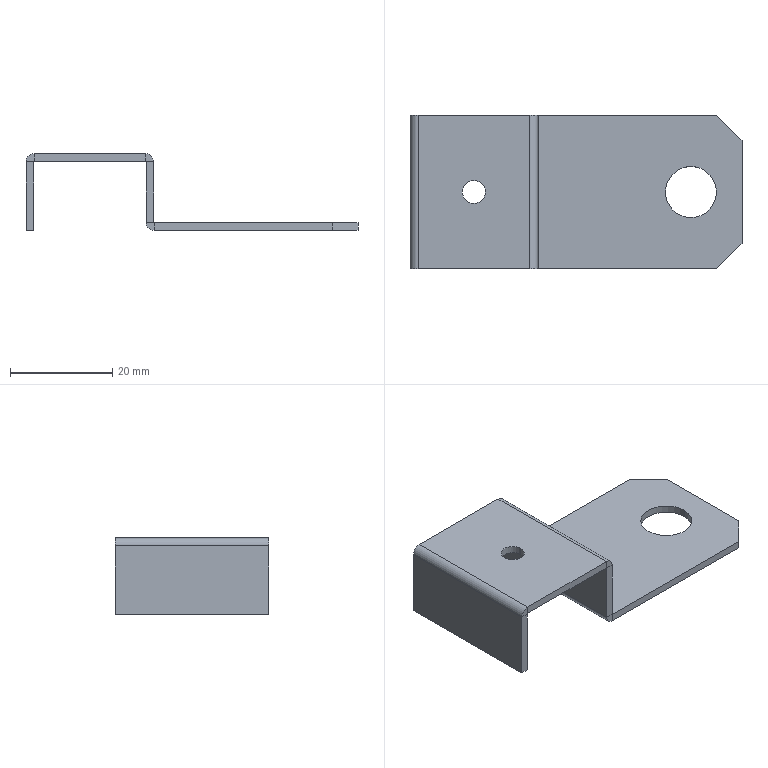Part | SolidWorks | features EdgeFlange 2, ICE 2, Chamfer 1, FlatPattern 1, SMBaseFlange 1, SheetMetal 1 | 1 solid | 36 faces | box 65 x 30 x 15 mm | volume 3912 mm3 | plane 26 | cylinder 10 | commonest cylinder face diameters 0.2 x3 3.2 x3 4.5 x2 10 x2
STEP:
#1=CARTESIAN_POINT('',(-2.25,0.,-1.5));
#2=VERTEX_POINT('',#1);
#3=CARTESIAN_POINT('',(2.25,0.,-1.5));
#4=VERTEX_POINT('',#3);
#5=CARTESIAN_POINT('',(0.,0.,-1.5));
#6=DIRECTION('',(0.,0.,1.));
#7=DIRECTION('',(1.,0.,0.));
#8=AXIS2_PLACEMENT_3D('',#5,#6,#7);
#9=CIRCLE('',#8,2.25);
#10=EDGE_CURVE('',#2,#4,#9,.T.);
#11=ORIENTED_EDGE('',*,*,#10,.F.);
#12=CARTESIAN_POINT('',(-2.25,0.,0.));
#13=VERTEX_POINT('',#12);
#14=CARTESIAN_POINT('',(-2.25,0.,-10.));
#15=DIRECTION('',(0.,0.,1.));
#16=VECTOR('',#15,1000.);
#17=LINE('',#14,#16);
#18=EDGE_CURVE('',#2,#13,#17,.T.);
#19=ORIENTED_EDGE('',*,*,#18,.T.);
#20=CARTESIAN_POINT('',(2.25,0.,0.));
#21=VERTEX_POINT('',#20);
#22=CARTESIAN_POINT('',(0.,0.,0.));
#23=DIRECTION('',(0.,0.,1.));
#24=DIRECTION('',(1.,0.,0.));
#25=AXIS2_PLACEMENT_3D('',#22,#23,#24);
#26=CIRCLE('',#25,2.25);
#27=EDGE_CURVE('',#13,#21,#26,.T.);
#28=ORIENTED_EDGE('',*,*,#27,.T.);
#29=CARTESIAN_POINT('',(2.25,0.,-10.));
#30=DIRECTION('',(0.,0.,1.));
#31=VECTOR('',#30,1000.);
#32=LINE('',#29,#31);
#33=EDGE_CURVE('',#4,#21,#32,.T.);
#34=ORIENTED_EDGE('',*,*,#33,.F.);
#35=EDGE_LOOP('',(#11,#19,#28,#34));
#36=FACE_OUTER_BOUND('',#35,.T.);
#37=CARTESIAN_POINT('',(0.,0.,-10.));
#38=DIRECTION('',(0.,0.,1.));
#39=DIRECTION('',(1.,0.,0.));
#40=AXIS2_PLACEMENT_3D('',#37,#38,#39);
#41=CYLINDRICAL_SURFACE('',#40,2.25);
#42=ADVANCED_FACE('',(#36),#41,.F.);
#43=CARTESIAN_POINT('',(37.5,0.,-15.));
#44=VERTEX_POINT('',#43);
#45=CARTESIAN_POINT('',(47.5,0.,-15.));
#46=VERTEX_POINT('',#45);
#47=CARTESIAN_POINT('',(42.5,0.,-15.));
#48=DIRECTION('',(0.,0.,1.));
#49=DIRECTION('',(1.,0.,0.));
#50=AXIS2_PLACEMENT_3D('',#47,#48,#49);
#51=CIRCLE('',#50,5.);
#52=EDGE_CURVE('',#44,#46,#51,.T.);
#53=ORIENTED_EDGE('',*,*,#52,.F.);
#54=CARTESIAN_POINT('',(37.5,0.,-13.5));
#55=VERTEX_POINT('',#54);
#56=CARTESIAN_POINT('',(37.5,0.,-23.5));
#57=DIRECTION('',(0.,0.,1.));
#58=VECTOR('',#57,1000.);
#59=LINE('',#56,#58);
#60=EDGE_CURVE('',#44,#55,#59,.T.);
#61=ORIENTED_EDGE('',*,*,#60,.T.);
#62=CARTESIAN_POINT('',(47.5,0.,-13.5));
#63=VERTEX_POINT('',#62);
#64=CARTESIAN_POINT('',(42.5,0.,-13.5));
#65=DIRECTION('',(0.,0.,1.));
#66=DIRECTION('',(1.,0.,0.));
#67=AXIS2_PLACEMENT_3D('',#64,#65,#66);
#68=CIRCLE('',#67,5.);
#69=EDGE_CURVE('',#55,#63,#68,.T.);
#70=ORIENTED_EDGE('',*,*,#69,.T.);
#71=CARTESIAN_POINT('',(47.5,0.,-23.5));
#72=DIRECTION('',(0.,0.,1.));
#73=VECTOR('',#72,1000.);
#74=LINE('',#71,#73);
#75=EDGE_CURVE('',#46,#63,#74,.T.);
#76=ORIENTED_EDGE('',*,*,#75,.F.);
#77=EDGE_LOOP('',(#53,#61,#70,#76));
#78=FACE_OUTER_BOUND('',#77,.T.);
#79=CARTESIAN_POINT('',(42.5,0.,-23.5));
#80=DIRECTION('',(0.,0.,1.));
#81=DIRECTION('',(1.,0.,0.));
#82=AXIS2_PLACEMENT_3D('',#79,#80,#81);
#83=CYLINDRICAL_SURFACE('',#82,5.);
#84=ADVANCED_FACE('',(#78),#83,.F.);
#85=CARTESIAN_POINT('',(12.5,-15.,-13.4));
#86=VERTEX_POINT('',#85);
#87=CARTESIAN_POINT('',(11.,-15.,-13.4));
#88=VERTEX_POINT('',#87);
#89=CARTESIAN_POINT('',(12.5,-15.,-13.4));
#90=DIRECTION('',(-1.,0.,0.));
#91=VECTOR('',#90,1000.);
#92=LINE('',#89,#91);
#93=EDGE_CURVE('',#86,#88,#92,.T.);
#94=ORIENTED_EDGE('',*,*,#93,.F.);
#95=CARTESIAN_POINT('',(12.5,-15.,-1.6));
#96=VERTEX_POINT('',#95);
#97=CARTESIAN_POINT('',(12.5,-15.,-1.5));
#98=DIRECTION('',(0.,0.,-1.));
#99=VECTOR('',#98,1000.);
#100=LINE('',#97,#99);
#101=EDGE_CURVE('',#96,#86,#100,.T.);
#102=ORIENTED_EDGE('',*,*,#101,.F.);
#103=CARTESIAN_POINT('',(11.,-15.,-1.6));
#104=VERTEX_POINT('',#103);
#105=CARTESIAN_POINT('',(11.,-15.,-1.6));
#106=DIRECTION('',(1.,0.,0.));
#107=VECTOR('',#106,1000.);
#108=LINE('',#105,#107);
#109=EDGE_CURVE('',#104,#96,#108,.T.);
#110=ORIENTED_EDGE('',*,*,#109,.F.);
#111=CARTESIAN_POINT('',(11.,-15.,-15.));
#112=DIRECTION('',(0.,0.,-1.));
#113=VECTOR('',#112,1000.);
#114=LINE('',#111,#113);
#115=EDGE_CURVE('',#104,#88,#114,.T.);
#116=ORIENTED_EDGE('',*,*,#115,.T.);
#117=EDGE_LOOP('',(#94,#102,#110,#116));
#118=FACE_OUTER_BOUND('',#117,.T.);
#119=CARTESIAN_POINT('',(12.5,-15.,-15.));
#120=DIRECTION('',(0.,1.,0.));
#121=DIRECTION('',(-1.,0.,0.));
#122=AXIS2_PLACEMENT_3D('',#119,#120,#121);
#123=PLANE('',#122);
#124=ADVANCED_FACE('',(#118),#123,.F.);
#125=CARTESIAN_POINT('',(12.5,15.,-13.4));
#126=VERTEX_POINT('',#125);
#127=CARTESIAN_POINT('',(11.,15.,-13.4));
#128=VERTEX_POINT('',#127);
#129=CARTESIAN_POINT('',(12.5,15.,-13.4));
#130=DIRECTION('',(-1.,0.,0.));
#131=VECTOR('',#130,1000.);
#132=LINE('',#129,#131);
#133=EDGE_CURVE('',#126,#128,#132,.T.);
#134=ORIENTED_EDGE('',*,*,#133,.T.);
#135=CARTESIAN_POINT('',(11.,15.,-1.6));
#136=VERTEX_POINT('',#135);
#137=CARTESIAN_POINT('',(11.,15.,-1.5));
#138=DIRECTION('',(0.,0.,1.));
#139=VECTOR('',#138,1000.);
#140=LINE('',#137,#139);
#141=EDGE_CURVE('',#128,#136,#140,.T.);
#142=ORIENTED_EDGE('',*,*,#141,.T.);
#143=CARTESIAN_POINT('',(12.5,15.,-1.6));
#144=VERTEX_POINT('',#143);
#145=CARTESIAN_POINT('',(12.5,15.,-1.6));
#146=DIRECTION('',(1.,0.,0.));
#147=VECTOR('',#146,1000.);
#148=LINE('',#145,#147);
#149=EDGE_CURVE('',#136,#144,#148,.T.);
#150=ORIENTED_EDGE('',*,*,#149,.T.);
#151=CARTESIAN_POINT('',(12.5,15.,-1.5));
#152=DIRECTION('',(0.,0.,1.));
#153=VECTOR('',#152,1000.);
#154=LINE('',#151,#153);
#155=EDGE_CURVE('',#126,#144,#154,.T.);
#156=ORIENTED_EDGE('',*,*,#155,.F.);
#157=EDGE_LOOP('',(#134,#142,#150,#156));
#158=FACE_OUTER_BOUND('',#157,.T.);
#159=CARTESIAN_POINT('',(12.5,15.,-1.5));
#160=DIRECTION('',(0.,-1.,0.));
#161=DIRECTION('',(1.,0.,0.));
#162=AXIS2_PLACEMENT_3D('',#159,#160,#161);
#163=PLANE('',#162);
#164=ADVANCED_FACE('',(#158),#163,.F.);
#165=CARTESIAN_POINT('',(12.5,15.,-13.4));
#166=DIRECTION('',(0.,-1.,0.));
#167=VECTOR('',#166,1000.);
#168=LINE('',#165,#167);
#169=EDGE_CURVE('',#126,#86,#168,.T.);
#170=ORIENTED_EDGE('',*,*,#169,.F.);
#171=ORIENTED_EDGE('',*,*,#155,.T.);
#172=CARTESIAN_POINT('',(12.5,15.,-1.6));
#173=DIRECTION('',(0.,1.,0.));
#174=VECTOR('',#173,1000.);
#175=LINE('',#172,#174);
#176=EDGE_CURVE('',#96,#144,#175,.T.);
#177=ORIENTED_EDGE('',*,*,#176,.F.);
#178=ORIENTED_EDGE('',*,*,#101,.T.);
#179=EDGE_LOOP('',(#170,#171,#177,#178));
#180=FACE_OUTER_BOUND('',#179,.T.);
#181=CARTESIAN_POINT('',(12.5,-15.,-1.5));
#182=DIRECTION('',(-1.,0.,0.));
#183=DIRECTION('',(0.,0.,1.));
#184=AXIS2_PLACEMENT_3D('',#181,#182,#183);
#185=PLANE('',#184);
#186=ADVANCED_FACE('',(#180),#185,.F.);
#187=ORIENTED_EDGE('',*,*,#141,.F.);
#188=CARTESIAN_POINT('',(11.,15.,-13.4));
#189=DIRECTION('',(0.,-1.,0.));
#190=VECTOR('',#189,1000.);
#191=LINE('',#188,#190);
#192=EDGE_CURVE('',#128,#88,#191,.T.);
#193=ORIENTED_EDGE('',*,*,#192,.T.);
#194=ORIENTED_EDGE('',*,*,#115,.F.);
#195=CARTESIAN_POINT('',(11.,15.,-1.6));
#196=DIRECTION('',(0.,-1.,0.));
#197=VECTOR('',#196,1000.);
#198=LINE('',#195,#197);
#199=EDGE_CURVE('',#136,#104,#198,.T.);
#200=ORIENTED_EDGE('',*,*,#199,.F.);
#201=EDGE_LOOP('',(#187,#193,#194,#200));
#202=FACE_OUTER_BOUND('',#201,.T.);
#203=CARTESIAN_POINT('',(11.,-15.,-1.5));
#204=DIRECTION('',(-1.,0.,0.));
#205=DIRECTION('',(0.,0.,1.));
#206=AXIS2_PLACEMENT_3D('',#203,#204,#205);
#207=PLANE('',#206);
#208=ADVANCED_FACE('',(#202),#207,.T.);
#209=CARTESIAN_POINT('',(0.,0.,-1.5));
#210=DIRECTION('',(0.,0.,1.));
#211=DIRECTION('',(1.,0.,0.));
#212=AXIS2_PLACEMENT_3D('',#209,#210,#211);
#213=CIRCLE('',#212,2.25);
#214=EDGE_CURVE('',#4,#2,#213,.T.);
#215=ORIENTED_EDGE('',*,*,#214,.T.);
#216=ORIENTED_EDGE('',*,*,#10,.T.);
#217=EDGE_LOOP('',(#215,#216));
#218=FACE_BOUND('',#217,.T.);
#219=CARTESIAN_POINT('',(-10.9,15.,-1.5));
#220=VERTEX_POINT('',#219);
#221=CARTESIAN_POINT('',(-10.9,-15.,-1.5));
#222=VERTEX_POINT('',#221);
#223=CARTESIAN_POINT('',(-10.9,15.,-1.5));
#224=DIRECTION('',(0.,-1.,0.));
#225=VECTOR('',#224,1000.);
#226=LINE('',#223,#225);
#227=EDGE_CURVE('',#220,#222,#226,.T.);
#228=ORIENTED_EDGE('',*,*,#227,.F.);
#229=CARTESIAN_POINT('',(10.9,15.,-1.5));
#230=VERTEX_POINT('',#229);
#231=CARTESIAN_POINT('',(-12.5,15.,-1.5));
#232=DIRECTION('',(-1.,0.,0.));
#233=VECTOR('',#232,1000.);
#234=LINE('',#231,#233);
#235=EDGE_CURVE('',#230,#220,#234,.T.);
#236=ORIENTED_EDGE('',*,*,#235,.F.);
#237=CARTESIAN_POINT('',(10.9,-15.,-1.5));
#238=VERTEX_POINT('',#237);
#239=CARTESIAN_POINT('',(10.9,-15.,-1.5));
#240=DIRECTION('',(0.,1.,0.));
#241=VECTOR('',#240,1000.);
#242=LINE('',#239,#241);
#243=EDGE_CURVE('',#238,#230,#242,.T.);
#244=ORIENTED_EDGE('',*,*,#243,.F.);
#245=CARTESIAN_POINT('',(-12.5,-15.,-1.5));
#246=DIRECTION('',(1.,0.,0.));
#247=VECTOR('',#246,1000.);
#248=LINE('',#245,#247);
#249=EDGE_CURVE('',#222,#238,#248,.T.);
#250=ORIENTED_EDGE('',*,*,#249,.F.);
#251=EDGE_LOOP('',(#228,#236,#244,#250));
#252=FACE_OUTER_BOUND('',#251,.T.);
#253=CARTESIAN_POINT('',(12.5,-15.,-1.5));
#254=DIRECTION('',(0.,0.,1.));
#255=DIRECTION('',(1.,0.,0.));
#256=AXIS2_PLACEMENT_3D('',#253,#254,#255);
#257=PLANE('',#256);
#258=ADVANCED_FACE('',(#218,#252),#257,.F.);
#259=CARTESIAN_POINT('',(0.,0.,0.));
#260=DIRECTION('',(0.,0.,1.));
#261=DIRECTION('',(1.,0.,0.));
#262=AXIS2_PLACEMENT_3D('',#259,#260,#261);
#263=CIRCLE('',#262,2.25);
#264=EDGE_CURVE('',#21,#13,#263,.T.);
#265=ORIENTED_EDGE('',*,*,#264,.F.);
#266=ORIENTED_EDGE('',*,*,#27,.F.);
#267=EDGE_LOOP('',(#265,#266));
#268=FACE_BOUND('',#267,.T.);
#269=CARTESIAN_POINT('',(10.9,15.,0.));
#270=VERTEX_POINT('',#269);
#271=CARTESIAN_POINT('',(-10.9,15.,0.));
#272=VERTEX_POINT('',#271);
#273=CARTESIAN_POINT('',(-12.5,15.,0.));
#274=DIRECTION('',(-1.,0.,0.));
#275=VECTOR('',#274,1000.);
#276=LINE('',#273,#275);
#277=EDGE_CURVE('',#270,#272,#276,.T.);
#278=ORIENTED_EDGE('',*,*,#277,.T.);
#279=CARTESIAN_POINT('',(-10.9,-15.,0.));
#280=VERTEX_POINT('',#279);
#281=CARTESIAN_POINT('',(-10.9,15.,0.));
#282=DIRECTION('',(0.,-1.,0.));
#283=VECTOR('',#282,1000.);
#284=LINE('',#281,#283);
#285=EDGE_CURVE('',#272,#280,#284,.T.);
#286=ORIENTED_EDGE('',*,*,#285,.T.);
#287=CARTESIAN_POINT('',(10.9,-15.,0.));
#288=VERTEX_POINT('',#287);
#289=CARTESIAN_POINT('',(-12.5,-15.,0.));
#290=DIRECTION('',(1.,0.,0.));
#291=VECTOR('',#290,1000.);
#292=LINE('',#289,#291);
#293=EDGE_CURVE('',#280,#288,#292,.T.);
#294=ORIENTED_EDGE('',*,*,#293,.T.);
#295=CARTESIAN_POINT('',(10.9,-15.,0.));
#296=DIRECTION('',(0.,1.,0.));
#297=VECTOR('',#296,1000.);
#298=LINE('',#295,#297);
#299=EDGE_CURVE('',#288,#270,#298,.T.);
#300=ORIENTED_EDGE('',*,*,#299,.T.);
#301=EDGE_LOOP('',(#278,#286,#294,#300));
#302=FACE_OUTER_BOUND('',#301,.T.);
#303=CARTESIAN_POINT('',(12.5,-15.,0.));
#304=DIRECTION('',(0.,0.,1.));
#305=DIRECTION('',(1.,0.,0.));
#306=AXIS2_PLACEMENT_3D('',#303,#304,#305);
#307=PLANE('',#306);
#308=ADVANCED_FACE('',(#268,#302),#307,.T.);
#309=ORIENTED_EDGE('',*,*,#235,.T.);
#310=CARTESIAN_POINT('',(-10.9,15.,-1.5));
#311=DIRECTION('',(0.,0.,1.));
#312=VECTOR('',#311,1000.);
#313=LINE('',#310,#312);
#314=EDGE_CURVE('',#220,#272,#313,.T.);
#315=ORIENTED_EDGE('',*,*,#314,.T.);
#316=ORIENTED_EDGE('',*,*,#277,.F.);
#317=CARTESIAN_POINT('',(10.9,15.,-1.5));
#318=DIRECTION('',(0.,0.,1.));
#319=VECTOR('',#318,1000.);
#320=LINE('',#317,#319);
#321=EDGE_CURVE('',#230,#270,#320,.T.);
#322=ORIENTED_EDGE('',*,*,#321,.F.);
#323=EDGE_LOOP('',(#309,#315,#316,#322));
#324=FACE_OUTER_BOUND('',#323,.T.);
#325=CARTESIAN_POINT('',(-12.5,15.,-1.5));
#326=DIRECTION('',(0.,1.,0.));
#327=DIRECTION('',(0.,0.,1.));
#328=AXIS2_PLACEMENT_3D('',#325,#326,#327);
#329=PLANE('',#328);
#330=ADVANCED_FACE('',(#324),#329,.T.);
#331=CARTESIAN_POINT('',(-10.9,-15.,-1.5));
#332=DIRECTION('',(0.,0.,1.));
#333=VECTOR('',#332,1000.);
#334=LINE('',#331,#333);
#335=EDGE_CURVE('',#222,#280,#334,.T.);
#336=ORIENTED_EDGE('',*,*,#335,.F.);
#337=ORIENTED_EDGE('',*,*,#249,.T.);
#338=CARTESIAN_POINT('',(10.9,-15.,-1.5));
#339=DIRECTION('',(0.,0.,1.));
#340=VECTOR('',#339,1000.);
#341=LINE('',#338,#340);
#342=EDGE_CURVE('',#238,#288,#341,.T.);
#343=ORIENTED_EDGE('',*,*,#342,.T.);
#344=ORIENTED_EDGE('',*,*,#293,.F.);
#345=EDGE_LOOP('',(#336,#337,#343,#344));
#346=FACE_OUTER_BOUND('',#345,.T.);
#347=CARTESIAN_POINT('',(-12.5,-15.,-1.5));
#348=DIRECTION('',(0.,-1.,0.));
#349=DIRECTION('',(0.,0.,-1.));
#350=AXIS2_PLACEMENT_3D('',#347,#348,#349);
#351=PLANE('',#350);
#352=ADVANCED_FACE('',(#346),#351,.T.);
#353=ORIENTED_EDGE('',*,*,#149,.F.);
#354=CARTESIAN_POINT('',(10.9,15.,-1.6));
#355=DIRECTION('',(0.,1.,0.));
#356=DIRECTION('',(0.,0.,-1.));
#357=AXIS2_PLACEMENT_3D('',#354,#355,#356);
#358=CIRCLE('',#357,0.1);
#359=EDGE_CURVE('',#230,#136,#358,.T.);
#360=ORIENTED_EDGE('',*,*,#359,.F.);
#361=ORIENTED_EDGE('',*,*,#321,.T.);
#362=CARTESIAN_POINT('',(10.9,15.,-1.6));
#363=DIRECTION('',(0.,1.,0.));
#364=DIRECTION('',(0.,0.,-1.));
#365=AXIS2_PLACEMENT_3D('',#362,#363,#364);
#366=CIRCLE('',#365,1.6);
#367=EDGE_CURVE('',#270,#144,#366,.T.);
#368=ORIENTED_EDGE('',*,*,#367,.T.);
#369=EDGE_LOOP('',(#353,#360,#361,#368));
#370=FACE_OUTER_BOUND('',#369,.T.);
#371=CARTESIAN_POINT('',(10.9,15.,-1.6));
#372=DIRECTION('',(0.,1.,0.));
#373=DIRECTION('',(0.,0.,1.));
#374=AXIS2_PLACEMENT_3D('',#371,#372,#373);
#375=PLANE('',#374);
#376=ADVANCED_FACE('',(#370),#375,.T.);
#377=CARTESIAN_POINT('',(10.9,-15.,-1.6));
#378=DIRECTION('',(0.,-1.,0.));
#379=DIRECTION('',(0.,0.,-1.));
#380=AXIS2_PLACEMENT_3D('',#377,#378,#379);
#381=CIRCLE('',#380,0.1);
#382=EDGE_CURVE('',#104,#238,#381,.T.);
#383=ORIENTED_EDGE('',*,*,#382,.F.);
#384=ORIENTED_EDGE('',*,*,#109,.T.);
#385=CARTESIAN_POINT('',(10.9,-15.,-1.6));
#386=DIRECTION('',(0.,-1.,0.));
#387=DIRECTION('',(0.,0.,-1.));
#388=AXIS2_PLACEMENT_3D('',#385,#386,#387);
#389=CIRCLE('',#388,1.6);
#390=EDGE_CURVE('',#96,#288,#389,.T.);
#391=ORIENTED_EDGE('',*,*,#390,.T.);
#392=ORIENTED_EDGE('',*,*,#342,.F.);
#393=EDGE_LOOP('',(#383,#384,#391,#392));
#394=FACE_OUTER_BOUND('',#393,.T.);
#395=CARTESIAN_POINT('',(10.9,-15.,-1.6));
#396=DIRECTION('',(0.,1.,0.));
#397=DIRECTION('',(0.,0.,1.));
#398=AXIS2_PLACEMENT_3D('',#395,#396,#397);
#399=PLANE('',#398);
#400=ADVANCED_FACE('',(#394),#399,.F.);
#401=ORIENTED_EDGE('',*,*,#299,.F.);
#402=ORIENTED_EDGE('',*,*,#390,.F.);
#403=ORIENTED_EDGE('',*,*,#176,.T.);
#404=ORIENTED_EDGE('',*,*,#367,.F.);
#405=EDGE_LOOP('',(#401,#402,#403,#404));
#406=FACE_OUTER_BOUND('',#405,.T.);
#407=CARTESIAN_POINT('',(10.9,-15.,-1.6));
#408=DIRECTION('',(0.,-1.,0.));
#409=DIRECTION('',(1.,0.,0.));
#410=AXIS2_PLACEMENT_3D('',#407,#408,#409);
#411=CYLINDRICAL_SURFACE('',#410,1.6);
#412=ADVANCED_FACE('',(#406),#411,.T.);
#413=ORIENTED_EDGE('',*,*,#243,.T.);
#414=ORIENTED_EDGE('',*,*,#359,.T.);
#415=ORIENTED_EDGE('',*,*,#199,.T.);
#416=ORIENTED_EDGE('',*,*,#382,.T.);
#417=EDGE_LOOP('',(#413,#414,#415,#416));
#418=FACE_OUTER_BOUND('',#417,.T.);
#419=CARTESIAN_POINT('',(10.9,-15.,-1.6));
#420=DIRECTION('',(0.,-1.,0.));
#421=DIRECTION('',(1.,0.,0.));
#422=AXIS2_PLACEMENT_3D('',#419,#420,#421);
#423=CYLINDRICAL_SURFACE('',#422,0.1);
#424=ADVANCED_FACE('',(#418),#423,.F.);
#425=CARTESIAN_POINT('',(-11.,-15.,-1.6));
#426=VERTEX_POINT('',#425);
#427=CARTESIAN_POINT('',(-12.5,-15.,-1.6));
#428=VERTEX_POINT('',#427);
#429=CARTESIAN_POINT('',(-12.5,-15.,-1.6));
#430=DIRECTION('',(-1.,0.,0.));
#431=VECTOR('',#430,1000.);
#432=LINE('',#429,#431);
#433=EDGE_CURVE('',#426,#428,#432,.T.);
#434=ORIENTED_EDGE('',*,*,#433,.F.);
#435=CARTESIAN_POINT('',(-10.9,-15.,-1.6));
#436=DIRECTION('',(0.,-1.,0.));
#437=DIRECTION('',(0.,0.,1.));
#438=AXIS2_PLACEMENT_3D('',#435,#436,#437);
#439=CIRCLE('',#438,0.1);
#440=EDGE_CURVE('',#222,#426,#439,.T.);
#441=ORIENTED_EDGE('',*,*,#440,.F.);
#442=ORIENTED_EDGE('',*,*,#335,.T.);
#443=CARTESIAN_POINT('',(-10.9,-15.,-1.6));
#444=DIRECTION('',(0.,-1.,0.));
#445=DIRECTION('',(0.,0.,1.));
#446=AXIS2_PLACEMENT_3D('',#443,#444,#445);
#447=CIRCLE('',#446,1.6);
#448=EDGE_CURVE('',#280,#428,#447,.T.);
#449=ORIENTED_EDGE('',*,*,#448,.T.);
#450=EDGE_LOOP('',(#434,#441,#442,#449));
#451=FACE_OUTER_BOUND('',#450,.T.);
#452=CARTESIAN_POINT('',(-10.9,-15.,-1.6));
#453=DIRECTION('',(0.,-1.,0.));
#454=DIRECTION('',(0.,0.,-1.));
#455=AXIS2_PLACEMENT_3D('',#452,#453,#454);
#456=PLANE('',#455);
#457=ADVANCED_FACE('',(#451),#456,.T.);
#458=CARTESIAN_POINT('',(-11.,15.,-1.6));
#459=VERTEX_POINT('',#458);
#460=CARTESIAN_POINT('',(-10.9,15.,-1.6));
#461=DIRECTION('',(0.,1.,0.));
#462=DIRECTION('',(0.,0.,1.));
#463=AXIS2_PLACEMENT_3D('',#460,#461,#462);
#464=CIRCLE('',#463,0.1);
#465=EDGE_CURVE('',#459,#220,#464,.T.);
#466=ORIENTED_EDGE('',*,*,#465,.F.);
#467=CARTESIAN_POINT('',(-12.5,15.,-1.6));
#468=VERTEX_POINT('',#467);
#469=CARTESIAN_POINT('',(-11.,15.,-1.6));
#470=DIRECTION('',(-1.,0.,0.));
#471=VECTOR('',#470,1000.);
#472=LINE('',#469,#471);
#473=EDGE_CURVE('',#459,#468,#472,.T.);
#474=ORIENTED_EDGE('',*,*,#473,.T.);
#475=CARTESIAN_POINT('',(-10.9,15.,-1.6));
#476=DIRECTION('',(0.,1.,0.));
#477=DIRECTION('',(0.,0.,1.));
#478=AXIS2_PLACEMENT_3D('',#475,#476,#477);
#479=CIRCLE('',#478,1.6);
#480=EDGE_CURVE('',#468,#272,#479,.T.);
#481=ORIENTED_EDGE('',*,*,#480,.T.);
#482=ORIENTED_EDGE('',*,*,#314,.F.);
#483=EDGE_LOOP('',(#466,#474,#481,#482));
#484=FACE_OUTER_BOUND('',#483,.T.);
#485=CARTESIAN_POINT('',(-10.9,15.,-1.6));
#486=DIRECTION('',(0.,-1.,0.));
#487=DIRECTION('',(0.,0.,-1.));
#488=AXIS2_PLACEMENT_3D('',#485,#486,#487);
#489=PLANE('',#488);
#490=ADVANCED_FACE('',(#484),#489,.F.);
#491=ORIENTED_EDGE('',*,*,#285,.F.);
#492=ORIENTED_EDGE('',*,*,#480,.F.);
#493=CARTESIAN_POINT('',(-12.5,-15.,-1.6));
#494=DIRECTION('',(0.,-1.,0.));
#495=VECTOR('',#494,1000.);
#496=LINE('',#493,#495);
#497=EDGE_CURVE('',#468,#428,#496,.T.);
#498=ORIENTED_EDGE('',*,*,#497,.T.);
#499=ORIENTED_EDGE('',*,*,#448,.F.);
#500=EDGE_LOOP('',(#491,#492,#498,#499));
#501=FACE_OUTER_BOUND('',#500,.T.);
#502=CARTESIAN_POINT('',(-10.9,15.,-1.6));
#503=DIRECTION('',(0.,1.,0.));
#504=DIRECTION('',(-1.,0.,0.));
#505=AXIS2_PLACEMENT_3D('',#502,#503,#504);
#506=CYLINDRICAL_SURFACE('',#505,1.6);
#507=ADVANCED_FACE('',(#501),#506,.T.);
#508=ORIENTED_EDGE('',*,*,#227,.T.);
#509=ORIENTED_EDGE('',*,*,#440,.T.);
#510=CARTESIAN_POINT('',(-11.,-15.,-1.6));
#511=DIRECTION('',(0.,1.,0.));
#512=VECTOR('',#511,1000.);
#513=LINE('',#510,#512);
#514=EDGE_CURVE('',#426,#459,#513,.T.);
#515=ORIENTED_EDGE('',*,*,#514,.T.);
#516=ORIENTED_EDGE('',*,*,#465,.T.);
#517=EDGE_LOOP('',(#508,#509,#515,#516));
#518=FACE_OUTER_BOUND('',#517,.T.);
#519=CARTESIAN_POINT('',(-10.9,15.,-1.6));
#520=DIRECTION('',(0.,1.,0.));
#521=DIRECTION('',(-1.,0.,0.));
#522=AXIS2_PLACEMENT_3D('',#519,#520,#521);
#523=CYLINDRICAL_SURFACE('',#522,0.1);
#524=ADVANCED_FACE('',(#518),#523,.F.);
#525=ORIENTED_EDGE('',*,*,#473,.F.);
#526=CARTESIAN_POINT('',(-11.,15.,-15.));
#527=VERTEX_POINT('',#526);
#528=CARTESIAN_POINT('',(-11.,15.,-15.));
#529=DIRECTION('',(0.,0.,-1.));
#530=VECTOR('',#529,1000.);
#531=LINE('',#528,#530);
#532=EDGE_CURVE('',#459,#527,#531,.T.);
#533=ORIENTED_EDGE('',*,*,#532,.T.);
#534=CARTESIAN_POINT('',(-12.5,15.,-15.));
#535=VERTEX_POINT('',#534);
#536=CARTESIAN_POINT('',(-12.5,15.,-15.));
#537=DIRECTION('',(1.,0.,0.));
#538=VECTOR('',#537,1000.);
#539=LINE('',#536,#538);
#540=EDGE_CURVE('',#535,#527,#539,.T.);
#541=ORIENTED_EDGE('',*,*,#540,.F.);
#542=CARTESIAN_POINT('',(-12.5,15.,-1.5));
#543=DIRECTION('',(0.,0.,-1.));
#544=VECTOR('',#543,1000.);
#545=LINE('',#542,#544);
#546=EDGE_CURVE('',#468,#535,#545,.T.);
#547=ORIENTED_EDGE('',*,*,#546,.F.);
#548=EDGE_LOOP('',(#525,#533,#541,#547));
#549=FACE_OUTER_BOUND('',#548,.T.);
#550=CARTESIAN_POINT('',(-12.5,15.,-15.));
#551=DIRECTION('',(0.,-1.,0.));
#552=DIRECTION('',(1.,0.,0.));
#553=AXIS2_PLACEMENT_3D('',#550,#551,#552);
#554=PLANE('',#553);
#555=ADVANCED_FACE('',(#549),#554,.F.);
#556=ORIENTED_EDGE('',*,*,#433,.T.);
#557=CARTESIAN_POINT('',(-12.5,-15.,-15.));
#558=VERTEX_POINT('',#557);
#559=CARTESIAN_POINT('',(-12.5,-15.,-1.5));
#560=DIRECTION('',(0.,0.,1.));
#561=VECTOR('',#560,1000.);
#562=LINE('',#559,#561);
#563=EDGE_CURVE('',#558,#428,#562,.T.);
#564=ORIENTED_EDGE('',*,*,#563,.F.);
#565=CARTESIAN_POINT('',(-11.,-15.,-15.));
#566=VERTEX_POINT('',#565);
#567=CARTESIAN_POINT('',(-12.5,-15.,-15.));
#568=DIRECTION('',(1.,0.,0.));
#569=VECTOR('',#568,1000.);
#570=LINE('',#567,#569);
#571=EDGE_CURVE('',#558,#566,#570,.T.);
#572=ORIENTED_EDGE('',*,*,#571,.T.);
#573=CARTESIAN_POINT('',(-11.,-15.,-1.5));
#574=DIRECTION('',(0.,0.,1.));
#575=VECTOR('',#574,1000.);
#576=LINE('',#573,#575);
#577=EDGE_CURVE('',#566,#426,#576,.T.);
#578=ORIENTED_EDGE('',*,*,#577,.T.);
#579=EDGE_LOOP('',(#556,#564,#572,#578));
#580=FACE_OUTER_BOUND('',#579,.T.);
#581=CARTESIAN_POINT('',(-12.5,-15.,-1.5));
#582=DIRECTION('',(0.,1.,0.));
#583=DIRECTION('',(-1.,0.,0.));
#584=AXIS2_PLACEMENT_3D('',#581,#582,#583);
#585=PLANE('',#584);
#586=ADVANCED_FACE('',(#580),#585,.F.);
#587=ORIENTED_EDGE('',*,*,#497,.F.);
#588=ORIENTED_EDGE('',*,*,#546,.T.);
#589=CARTESIAN_POINT('',(-12.5,15.,-15.));
#590=DIRECTION('',(0.,-1.,0.));
#591=VECTOR('',#590,1000.);
#592=LINE('',#589,#591);
#593=EDGE_CURVE('',#535,#558,#592,.T.);
#594=ORIENTED_EDGE('',*,*,#593,.T.);
#595=ORIENTED_EDGE('',*,*,#563,.T.);
#596=EDGE_LOOP('',(#587,#588,#594,#595));
#597=FACE_OUTER_BOUND('',#596,.T.);
#598=CARTESIAN_POINT('',(-12.5,15.,-1.5));
#599=DIRECTION('',(1.,0.,0.));
#600=DIRECTION('',(0.,0.,-1.));
#601=AXIS2_PLACEMENT_3D('',#598,#599,#600);
#602=PLANE('',#601);
#603=ADVANCED_FACE('',(#597),#602,.F.);
#604=ORIENTED_EDGE('',*,*,#532,.F.);
#605=ORIENTED_EDGE('',*,*,#514,.F.);
#606=ORIENTED_EDGE('',*,*,#577,.F.);
#607=CARTESIAN_POINT('',(-11.,-15.,-15.));
#608=DIRECTION('',(0.,-1.,0.));
#609=VECTOR('',#608,1000.);
#610=LINE('',#607,#609);
#611=EDGE_CURVE('',#527,#566,#610,.T.);
#612=ORIENTED_EDGE('',*,*,#611,.F.);
#613=EDGE_LOOP('',(#604,#605,#606,#612));
#614=FACE_OUTER_BOUND('',#613,.T.);
#615=CARTESIAN_POINT('',(-11.,15.,-1.5));
#616=DIRECTION('',(1.,0.,0.));
#617=DIRECTION('',(0.,0.,-1.));
#618=AXIS2_PLACEMENT_3D('',#615,#616,#617);
#619=PLANE('',#618);
#620=ADVANCED_FACE('',(#614),#619,.T.);
#621=ORIENTED_EDGE('',*,*,#611,.T.);
#622=ORIENTED_EDGE('',*,*,#571,.F.);
#623=ORIENTED_EDGE('',*,*,#593,.F.);
#624=ORIENTED_EDGE('',*,*,#540,.T.);
#625=EDGE_LOOP('',(#621,#622,#623,#624));
#626=FACE_OUTER_BOUND('',#625,.T.);
#627=CARTESIAN_POINT('',(-12.5,-15.,-15.));
#628=DIRECTION('',(0.,0.,1.));
#629=DIRECTION('',(1.,0.,0.));
#630=AXIS2_PLACEMENT_3D('',#627,#628,#629);
#631=PLANE('',#630);
#632=ADVANCED_FACE('',(#626),#631,.F.);
#633=CARTESIAN_POINT('',(12.6,-15.,-13.5));
#634=VERTEX_POINT('',#633);
#635=CARTESIAN_POINT('',(12.6,-15.,-15.));
#636=VERTEX_POINT('',#635);
#637=CARTESIAN_POINT('',(12.6,-15.,-15.));
#638=DIRECTION('',(0.,0.,-1.));
#639=VECTOR('',#638,1000.);
#640=LINE('',#637,#639);
#641=EDGE_CURVE('',#634,#636,#640,.T.);
#642=ORIENTED_EDGE('',*,*,#641,.F.);
#643=CARTESIAN_POINT('',(12.6,-15.,-13.4));
#644=DIRECTION('',(0.,-1.,0.));
#645=DIRECTION('',(0.,0.,1.));
#646=AXIS2_PLACEMENT_3D('',#643,#644,#645);
#647=CIRCLE('',#646,0.1);
#648=EDGE_CURVE('',#86,#634,#647,.T.);
#649=ORIENTED_EDGE('',*,*,#648,.F.);
#650=ORIENTED_EDGE('',*,*,#93,.T.);
#651=CARTESIAN_POINT('',(12.6,-15.,-13.4));
#652=DIRECTION('',(0.,-1.,0.));
#653=DIRECTION('',(0.,0.,1.));
#654=AXIS2_PLACEMENT_3D('',#651,#652,#653);
#655=CIRCLE('',#654,1.6);
#656=EDGE_CURVE('',#88,#636,#655,.T.);
#657=ORIENTED_EDGE('',*,*,#656,.T.);
#658=EDGE_LOOP('',(#642,#649,#650,#657));
#659=FACE_OUTER_BOUND('',#658,.T.);
#660=CARTESIAN_POINT('',(12.6,-15.,-13.4));
#661=DIRECTION('',(0.,-1.,0.));
#662=DIRECTION('',(0.,0.,-1.));
#663=AXIS2_PLACEMENT_3D('',#660,#661,#662);
#664=PLANE('',#663);
#665=ADVANCED_FACE('',(#659),#664,.T.);
#666=CARTESIAN_POINT('',(12.6,15.,-13.5));
#667=VERTEX_POINT('',#666);
#668=CARTESIAN_POINT('',(12.6,15.,-13.4));
#669=DIRECTION('',(0.,1.,0.));
#670=DIRECTION('',(0.,0.,1.));
#671=AXIS2_PLACEMENT_3D('',#668,#669,#670);
#672=CIRCLE('',#671,0.1);
#673=EDGE_CURVE('',#667,#126,#672,.T.);
#674=ORIENTED_EDGE('',*,*,#673,.F.);
#675=CARTESIAN_POINT('',(12.6,15.,-15.));
#676=VERTEX_POINT('',#675);
#677=CARTESIAN_POINT('',(12.6,15.,-13.5));
#678=DIRECTION('',(0.,0.,-1.));
#679=VECTOR('',#678,1000.);
#680=LINE('',#677,#679);
#681=EDGE_CURVE('',#667,#676,#680,.T.);
#682=ORIENTED_EDGE('',*,*,#681,.T.);
#683=CARTESIAN_POINT('',(12.6,15.,-13.4));
#684=DIRECTION('',(0.,1.,0.));
#685=DIRECTION('',(0.,0.,1.));
#686=AXIS2_PLACEMENT_3D('',#683,#684,#685);
#687=CIRCLE('',#686,1.6);
#688=EDGE_CURVE('',#676,#128,#687,.T.);
#689=ORIENTED_EDGE('',*,*,#688,.T.);
#690=ORIENTED_EDGE('',*,*,#133,.F.);
#691=EDGE_LOOP('',(#674,#682,#689,#690));
#692=FACE_OUTER_BOUND('',#691,.T.);
#693=CARTESIAN_POINT('',(12.6,15.,-13.4));
#694=DIRECTION('',(0.,-1.,0.));
#695=DIRECTION('',(0.,0.,-1.));
#696=AXIS2_PLACEMENT_3D('',#693,#694,#695);
#697=PLANE('',#696);
#698=ADVANCED_FACE('',(#692),#697,.F.);
#699=ORIENTED_EDGE('',*,*,#192,.F.);
#700=ORIENTED_EDGE('',*,*,#688,.F.);
#701=CARTESIAN_POINT('',(12.6,-15.,-15.));
#702=DIRECTION('',(0.,-1.,0.));
#703=VECTOR('',#702,1000.);
#704=LINE('',#701,#703);
#705=EDGE_CURVE('',#676,#636,#704,.T.);
#706=ORIENTED_EDGE('',*,*,#705,.T.);
#707=ORIENTED_EDGE('',*,*,#656,.F.);
#708=EDGE_LOOP('',(#699,#700,#706,#707));
#709=FACE_OUTER_BOUND('',#708,.T.);
#710=CARTESIAN_POINT('',(12.6,15.,-13.4));
#711=DIRECTION('',(0.,1.,0.));
#712=DIRECTION('',(0.,0.,-1.));
#713=AXIS2_PLACEMENT_3D('',#710,#711,#712);
#714=CYLINDRICAL_SURFACE('',#713,1.6);
#715=ADVANCED_FACE('',(#709),#714,.T.);
#716=ORIENTED_EDGE('',*,*,#169,.T.);
#717=ORIENTED_EDGE('',*,*,#648,.T.);
#718=CARTESIAN_POINT('',(12.6,-15.,-13.5));
#719=DIRECTION('',(0.,1.,0.));
#720=VECTOR('',#719,1000.);
#721=LINE('',#718,#720);
#722=EDGE_CURVE('',#634,#667,#721,.T.);
#723=ORIENTED_EDGE('',*,*,#722,.T.);
#724=ORIENTED_EDGE('',*,*,#673,.T.);
#725=EDGE_LOOP('',(#716,#717,#723,#724));
#726=FACE_OUTER_BOUND('',#725,.T.);
#727=CARTESIAN_POINT('',(12.6,15.,-13.4));
#728=DIRECTION('',(0.,1.,0.));
#729=DIRECTION('',(0.,0.,-1.));
#730=AXIS2_PLACEMENT_3D('',#727,#728,#729);
#731=CYLINDRICAL_SURFACE('',#730,0.1);
#732=ADVANCED_FACE('',(#726),#731,.F.);
#733=CARTESIAN_POINT('',(47.5,-15.,-15.));
#734=VERTEX_POINT('',#733);
#735=CARTESIAN_POINT('',(52.5,-15.,-15.));
#736=DIRECTION('',(-1.,0.,0.));
#737=VECTOR('',#736,1000.);
#738=LINE('',#735,#737);
#739=EDGE_CURVE('',#734,#636,#738,.T.);
#740=ORIENTED_EDGE('',*,*,#739,.F.);
#741=CARTESIAN_POINT('',(47.5,-15.,-13.5));
#742=VERTEX_POINT('',#741);
#743=CARTESIAN_POINT('',(47.5,-15.,-15.));
#744=DIRECTION('',(0.,0.,1.));
#745=VECTOR('',#744,1000.);
#746=LINE('',#743,#745);
#747=EDGE_CURVE('',#734,#742,#746,.T.);
#748=ORIENTED_EDGE('',*,*,#747,.T.);
#749=CARTESIAN_POINT('',(12.5,-15.,-13.5));
#750=DIRECTION('',(-1.,0.,0.));
#751=VECTOR('',#750,1000.);
#752=LINE('',#749,#751);
#753=EDGE_CURVE('',#742,#634,#752,.T.);
#754=ORIENTED_EDGE('',*,*,#753,.T.);
#755=ORIENTED_EDGE('',*,*,#641,.T.);
#756=EDGE_LOOP('',(#740,#748,#754,#755));
#757=FACE_OUTER_BOUND('',#756,.T.);
#758=CARTESIAN_POINT('',(12.5,-15.,-15.));
#759=DIRECTION('',(0.,1.,0.));
#760=DIRECTION('',(-1.,0.,0.));
#761=AXIS2_PLACEMENT_3D('',#758,#759,#760);
#762=PLANE('',#761);
#763=ADVANCED_FACE('',(#757),#762,.F.);
#764=CARTESIAN_POINT('',(47.5,15.,-13.5));
#765=VERTEX_POINT('',#764);
#766=CARTESIAN_POINT('',(52.5,15.,-13.5));
#767=DIRECTION('',(1.,0.,0.));
#768=VECTOR('',#767,1000.);
#769=LINE('',#766,#768);
#770=EDGE_CURVE('',#667,#765,#769,.T.);
#771=ORIENTED_EDGE('',*,*,#770,.T.);
#772=CARTESIAN_POINT('',(47.5,15.,-15.));
#773=VERTEX_POINT('',#772);
#774=CARTESIAN_POINT('',(47.5,15.,-15.));
#775=DIRECTION('',(0.,0.,-1.));
#776=VECTOR('',#775,1000.);
#777=LINE('',#774,#776);
#778=EDGE_CURVE('',#765,#773,#777,.T.);
#779=ORIENTED_EDGE('',*,*,#778,.T.);
#780=CARTESIAN_POINT('',(52.5,15.,-15.));
#781=DIRECTION('',(1.,0.,0.));
#782=VECTOR('',#781,1000.);
#783=LINE('',#780,#782);
#784=EDGE_CURVE('',#676,#773,#783,.T.);
#785=ORIENTED_EDGE('',*,*,#784,.F.);
#786=ORIENTED_EDGE('',*,*,#681,.F.);
#787=EDGE_LOOP('',(#771,#779,#785,#786));
#788=FACE_OUTER_BOUND('',#787,.T.);
#789=CARTESIAN_POINT('',(52.5,15.,-15.));
#790=DIRECTION('',(0.,-1.,0.));
#791=DIRECTION('',(1.,0.,0.));
#792=AXIS2_PLACEMENT_3D('',#789,#790,#791);
#793=PLANE('',#792);
#794=ADVANCED_FACE('',(#788),#793,.F.);
#795=CARTESIAN_POINT('',(42.5,0.,-15.));
#796=DIRECTION('',(0.,0.,1.));
#797=DIRECTION('',(1.,0.,0.));
#798=AXIS2_PLACEMENT_3D('',#795,#796,#797);
#799=CIRCLE('',#798,5.);
#800=EDGE_CURVE('',#46,#44,#799,.T.);
#801=ORIENTED_EDGE('',*,*,#800,.T.);
#802=ORIENTED_EDGE('',*,*,#52,.T.);
#803=EDGE_LOOP('',(#801,#802));
#804=FACE_BOUND('',#803,.T.);
#805=CARTESIAN_POINT('',(52.5,10.,-15.));
#806=VERTEX_POINT('',#805);
#807=CARTESIAN_POINT('',(52.5,-10.,-15.));
#808=VERTEX_POINT('',#807);
#809=CARTESIAN_POINT('',(52.5,-15.,-15.));
#810=DIRECTION('',(0.,-1.,0.));
#811=VECTOR('',#810,1000.);
#812=LINE('',#809,#811);
#813=EDGE_CURVE('',#806,#808,#812,.T.);
#814=ORIENTED_EDGE('',*,*,#813,.T.);
#815=CARTESIAN_POINT('',(47.5,-15.,-15.));
#816=DIRECTION('',(-0.7071,-0.7071,0.));
#817=VECTOR('',#816,1000.);
#818=LINE('',#815,#817);
#819=EDGE_CURVE('',#808,#734,#818,.T.);
#820=ORIENTED_EDGE('',*,*,#819,.T.);
#821=ORIENTED_EDGE('',*,*,#739,.T.);
#822=ORIENTED_EDGE('',*,*,#705,.F.);
#823=ORIENTED_EDGE('',*,*,#784,.T.);
#824=CARTESIAN_POINT('',(52.5,10.,-15.));
#825=DIRECTION('',(0.7071,-0.7071,0.));
#826=VECTOR('',#825,1000.);
#827=LINE('',#824,#826);
#828=EDGE_CURVE('',#773,#806,#827,.T.);
#829=ORIENTED_EDGE('',*,*,#828,.T.);
#830=EDGE_LOOP('',(#814,#820,#821,#822,#823,#829));
#831=FACE_OUTER_BOUND('',#830,.T.);
#832=CARTESIAN_POINT('',(52.5,-15.,-15.));
#833=DIRECTION('',(0.,0.,1.));
#834=DIRECTION('',(1.,0.,0.));
#835=AXIS2_PLACEMENT_3D('',#832,#833,#834);
#836=PLANE('',#835);
#837=ADVANCED_FACE('',(#804,#831),#836,.F.);
#838=CARTESIAN_POINT('',(42.5,0.,-13.5));
#839=DIRECTION('',(0.,0.,1.));
#840=DIRECTION('',(1.,0.,0.));
#841=AXIS2_PLACEMENT_3D('',#838,#839,#840);
#842=CIRCLE('',#841,5.);
#843=EDGE_CURVE('',#63,#55,#842,.T.);
#844=ORIENTED_EDGE('',*,*,#843,.F.);
#845=ORIENTED_EDGE('',*,*,#69,.F.);
#846=EDGE_LOOP('',(#844,#845));
#847=FACE_BOUND('',#846,.T.);
#848=ORIENTED_EDGE('',*,*,#753,.F.);
#849=CARTESIAN_POINT('',(52.5,-10.,-13.5));
#850=VERTEX_POINT('',#849);
#851=CARTESIAN_POINT('',(50.,-12.5,-13.5));
#852=DIRECTION('',(0.7071,0.7071,0.));
#853=VECTOR('',#852,1000.);
#854=LINE('',#851,#853);
#855=EDGE_CURVE('',#742,#850,#854,.T.);
#856=ORIENTED_EDGE('',*,*,#855,.T.);
#857=CARTESIAN_POINT('',(52.5,10.,-13.5));
#858=VERTEX_POINT('',#857);
#859=CARTESIAN_POINT('',(52.5,-15.,-13.5));
#860=DIRECTION('',(0.,-1.,0.));
#861=VECTOR('',#860,1000.);
#862=LINE('',#859,#861);
#863=EDGE_CURVE('',#858,#850,#862,.T.);
#864=ORIENTED_EDGE('',*,*,#863,.F.);
#865=CARTESIAN_POINT('',(65.,-2.5,-13.5));
#866=DIRECTION('',(-0.7071,0.7071,0.));
#867=VECTOR('',#866,1000.);
#868=LINE('',#865,#867);
#869=EDGE_CURVE('',#858,#765,#868,.T.);
#870=ORIENTED_EDGE('',*,*,#869,.T.);
#871=ORIENTED_EDGE('',*,*,#770,.F.);
#872=ORIENTED_EDGE('',*,*,#722,.F.);
#873=EDGE_LOOP('',(#848,#856,#864,#870,#871,#872));
#874=FACE_OUTER_BOUND('',#873,.T.);
#875=CARTESIAN_POINT('',(52.5,-15.,-13.5));
#876=DIRECTION('',(0.,0.,1.));
#877=DIRECTION('',(1.,0.,0.));
#878=AXIS2_PLACEMENT_3D('',#875,#876,#877);
#879=PLANE('',#878);
#880=ADVANCED_FACE('',(#847,#874),#879,.T.);
#881=ORIENTED_EDGE('',*,*,#863,.T.);
#882=CARTESIAN_POINT('',(52.5,-10.,-15.));
#883=DIRECTION('',(0.,0.,-1.));
#884=VECTOR('',#883,1000.);
#885=LINE('',#882,#884);
#886=EDGE_CURVE('',#850,#808,#885,.T.);
#887=ORIENTED_EDGE('',*,*,#886,.T.);
#888=ORIENTED_EDGE('',*,*,#813,.F.);
#889=CARTESIAN_POINT('',(52.5,10.,-15.));
#890=DIRECTION('',(0.,0.,1.));
#891=VECTOR('',#890,1000.);
#892=LINE('',#889,#891);
#893=EDGE_CURVE('',#806,#858,#892,.T.);
#894=ORIENTED_EDGE('',*,*,#893,.T.);
#895=EDGE_LOOP('',(#881,#887,#888,#894));
#896=FACE_OUTER_BOUND('',#895,.T.);
#897=CARTESIAN_POINT('',(52.5,-15.,-15.));
#898=DIRECTION('',(-1.,0.,0.));
#899=DIRECTION('',(0.,0.,1.));
#900=AXIS2_PLACEMENT_3D('',#897,#898,#899);
#901=PLANE('',#900);
#902=ADVANCED_FACE('',(#896),#901,.F.);
#903=ORIENTED_EDGE('',*,*,#819,.F.);
#904=ORIENTED_EDGE('',*,*,#886,.F.);
#905=ORIENTED_EDGE('',*,*,#855,.F.);
#906=ORIENTED_EDGE('',*,*,#747,.F.);
#907=EDGE_LOOP('',(#903,#904,#905,#906));
#908=FACE_OUTER_BOUND('',#907,.T.);
#909=CARTESIAN_POINT('',(47.5,-15.,-15.));
#910=DIRECTION('',(-0.7071,0.7071,0.));
#911=DIRECTION('',(-0.7071,-0.7071,0.));
#912=AXIS2_PLACEMENT_3D('',#909,#910,#911);
#913=PLANE('',#912);
#914=ADVANCED_FACE('',(#908),#913,.F.);
#915=ORIENTED_EDGE('',*,*,#828,.F.);
#916=ORIENTED_EDGE('',*,*,#778,.F.);
#917=ORIENTED_EDGE('',*,*,#869,.F.);
#918=ORIENTED_EDGE('',*,*,#893,.F.);
#919=EDGE_LOOP('',(#915,#916,#917,#918));
#920=FACE_OUTER_BOUND('',#919,.T.);
#921=CARTESIAN_POINT('',(52.5,10.,-15.));
#922=DIRECTION('',(-0.7071,-0.7071,0.));
#923=DIRECTION('',(0.7071,-0.7071,0.));
#924=AXIS2_PLACEMENT_3D('',#921,#922,#923);
#925=PLANE('',#924);
#926=ADVANCED_FACE('',(#920),#925,.F.);
#927=ORIENTED_EDGE('',*,*,#60,.F.);
#928=ORIENTED_EDGE('',*,*,#800,.F.);
#929=ORIENTED_EDGE('',*,*,#75,.T.);
#930=ORIENTED_EDGE('',*,*,#843,.T.);
#931=EDGE_LOOP('',(#927,#928,#929,#930));
#932=FACE_OUTER_BOUND('',#931,.T.);
#933=CARTESIAN_POINT('',(42.5,0.,-23.5));
#934=DIRECTION('',(0.,0.,1.));
#935=DIRECTION('',(1.,0.,0.));
#936=AXIS2_PLACEMENT_3D('',#933,#934,#935);
#937=CYLINDRICAL_SURFACE('',#936,5.);
#938=ADVANCED_FACE('',(#932),#937,.F.);
#939=ORIENTED_EDGE('',*,*,#18,.F.);
#940=ORIENTED_EDGE('',*,*,#214,.F.);
#941=ORIENTED_EDGE('',*,*,#33,.T.);
#942=ORIENTED_EDGE('',*,*,#264,.T.);
#943=EDGE_LOOP('',(#939,#940,#941,#942));
#944=FACE_OUTER_BOUND('',#943,.T.);
#945=CARTESIAN_POINT('',(0.,0.,-10.));
#946=DIRECTION('',(0.,0.,1.));
#947=DIRECTION('',(1.,0.,0.));
#948=AXIS2_PLACEMENT_3D('',#945,#946,#947);
#949=CYLINDRICAL_SURFACE('',#948,2.25);
#950=ADVANCED_FACE('',(#944),#949,.F.);
#951=CLOSED_SHELL('',(#42,#84,#124,#164,#186,#208,#258,#308,#330,#352,#376,#400,#412,#424,#457,#490,#507,#524,#555,#586,#603,#620,#632,#665,#698,#715,#732,#763,#794,#837,#880,#902,#914,#926,#938,#950));
#952=MANIFOLD_SOLID_BREP('',#951);
#953=CARTESIAN_POINT('',(0.,0.,0.));
#954=DIRECTION('',(0.,0.,1.));
#955=DIRECTION('',(1.,0.,0.));
#956=AXIS2_PLACEMENT_3D('',#953,#954,#955);
#957=(LENGTH_UNIT()NAMED_UNIT(*)SI_UNIT(.MILLI.,.METRE.));
#958=UNCERTAINTY_MEASURE_WITH_UNIT(LENGTH_MEASURE(0.00001),#957,'','');
#959=(NAMED_UNIT(*)PLANE_ANGLE_UNIT()SI_UNIT($,.RADIAN.));
#960=(NAMED_UNIT(*)SI_UNIT($,.STERADIAN.)SOLID_ANGLE_UNIT());
#961=(GEOMETRIC_REPRESENTATION_CONTEXT(3)GLOBAL_UNCERTAINTY_ASSIGNED_CONTEXT((#958))GLOBAL_UNIT_ASSIGNED_CONTEXT((#957,#959,#960))REPRESENTATION_CONTEXT('',''));
#962=ADVANCED_BREP_SHAPE_REPRESENTATION('',(#952,#956),#961);